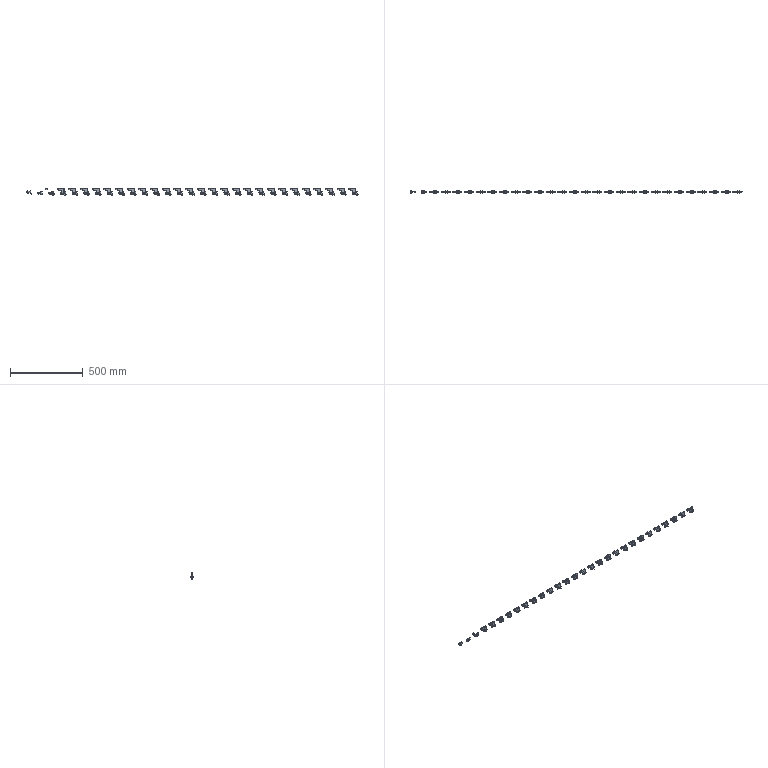Part | NX | 282 solids | 6470 faces | volume 276325 mm3 | plane 4033 | cylinder 2227 | cone 210 | commonest cylinder face diameters 3 x796 4 x662 5.1 x232 3.3 x156 7 x116 4.2 x104